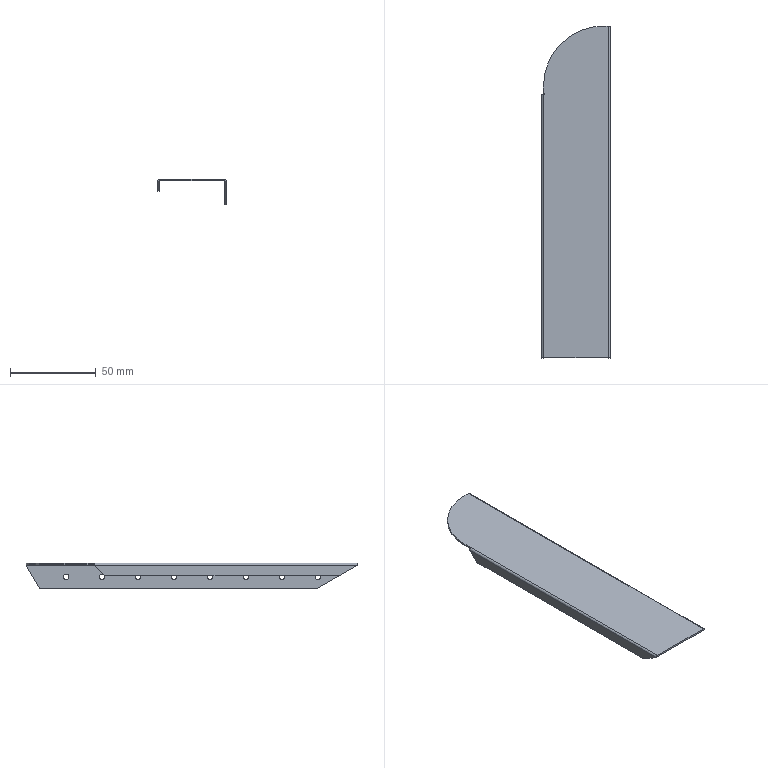Part | STEP file | HESS-408-70-15W-N-16-inner liner louver left side panel | 1 solid | 39 faces | box 40 x 194 x 15 mm | volume 10672 mm3 | cylinder 21 | plane 18 | commonest cylinder face diameters 3.2 x16 0.2 x2 2.2 x2 70 x1